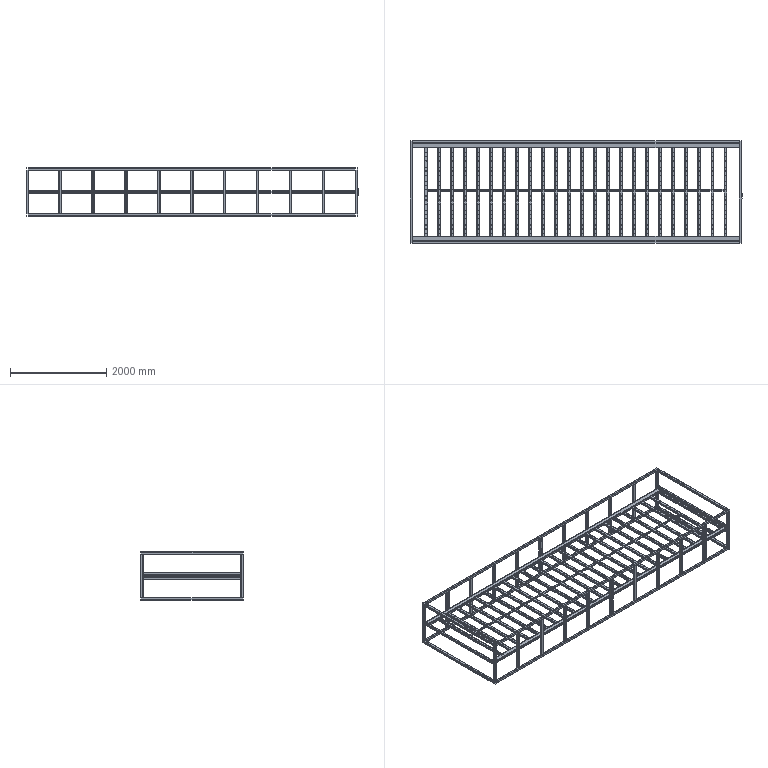Part | SolidWorks | features WeldCornerFeat 13, LPattern 7, HoleWzd 5, ICE 5, MoveCopyBody 4, WeldMemberFeat 4, 3DProfileFeature 1, Cut 1, MirrorSolid 1, WeldmentFeature 1 | 101 solids | 4708 faces | volume 76543847 mm3 | cylinder 3694 | plane 1002 | cone 12 | commonest cylinder face diameters 4.2 x1728 6.8 x580 15.5 x576 12 x292 6 x288 4 x92